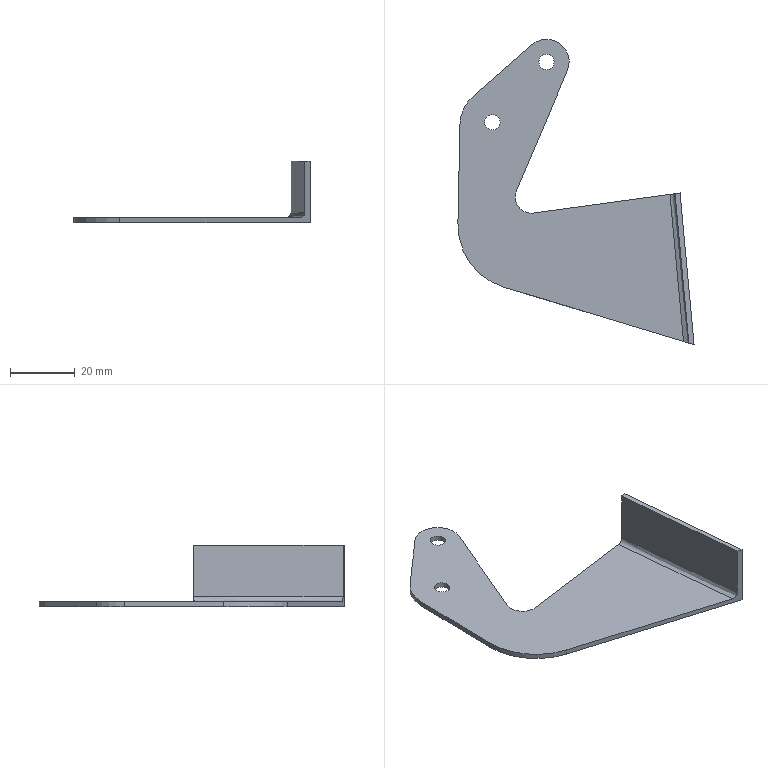Part | NX | features door hinge 2(left) 2 | 1 solid | 17 faces | box 72.898 x 94.256 x 19 mm | volume 6455 mm3 | plane 8 | cylinder 6 | spline 3 | commonest cylinder face diameters 4.762 x1 4.763 x1 10 x1 14 x1 24 x1 40 x1
STEP:
#1=CARTESIAN_POINT('',(6.443,-2.735,1.575));
#2=VERTEX_POINT('',#1);
#3=CARTESIAN_POINT('',(6.443,-2.735,0.));
#4=VERTEX_POINT('',#3);
#5=CARTESIAN_POINT('',(6.443,-2.735,19.));
#6=DIRECTION('',(0.,0.,-1.));
#7=VECTOR('',#6,1000.);
#8=LINE('',#5,#7);
#9=EDGE_CURVE('',#2,#4,#8,.T.);
#10=ORIENTED_EDGE('',*,*,#9,.T.);
#11=CARTESIAN_POINT('',(-4.613,5.265,0.));
#12=VERTEX_POINT('',#11);
#13=CARTESIAN_POINT('',(0.,0.,0.));
#14=DIRECTION('',(0.,0.,1.));
#15=DIRECTION('',(1.,0.,0.));
#16=AXIS2_PLACEMENT_3D('',#13,#14,#15);
#17=CIRCLE('',#16,7.);
#18=EDGE_CURVE('',#4,#12,#17,.T.);
#19=ORIENTED_EDGE('',*,*,#18,.T.);
#20=CARTESIAN_POINT('',(-4.613,5.265,1.575));
#21=VERTEX_POINT('',#20);
#22=CARTESIAN_POINT('',(-4.613,5.265,19.));
#23=DIRECTION('',(0.,0.,-1.));
#24=VECTOR('',#23,1000.);
#25=LINE('',#22,#24);
#26=EDGE_CURVE('',#21,#12,#25,.T.);
#27=ORIENTED_EDGE('',*,*,#26,.F.);
#28=CARTESIAN_POINT('',(0.,0.,1.575));
#29=DIRECTION('',(0.,0.,1.));
#30=DIRECTION('',(1.,0.,0.));
#31=AXIS2_PLACEMENT_3D('',#28,#29,#30);
#32=CIRCLE('',#31,7.);
#33=EDGE_CURVE('',#2,#21,#32,.T.);
#34=ORIENTED_EDGE('',*,*,#33,.F.);
#35=EDGE_LOOP('',(#10,#19,#27,#34));
#36=FACE_BOUND('',#35,.T.);
#37=CARTESIAN_POINT('',(0.,0.,19.));
#38=DIRECTION('',(0.,0.,-1.));
#39=DIRECTION('',(1.,0.,0.));
#40=AXIS2_PLACEMENT_3D('',#37,#38,#39);
#41=CYLINDRICAL_SURFACE('',#40,7.);
#42=ADVANCED_FACE('',(#36),#41,.T.);
#43=CARTESIAN_POINT('',(-9.254,-39.713,1.575));
#44=VERTEX_POINT('',#43);
#45=CARTESIAN_POINT('',(-9.254,-39.713,0.));
#46=VERTEX_POINT('',#45);
#47=CARTESIAN_POINT('',(-9.254,-39.713,19.));
#48=DIRECTION('',(0.,0.,-1.));
#49=VECTOR('',#48,1000.);
#50=LINE('',#47,#49);
#51=EDGE_CURVE('',#44,#46,#50,.T.);
#52=ORIENTED_EDGE('',*,*,#51,.T.);
#53=CARTESIAN_POINT('',(6.443,-2.735,0.));
#54=DIRECTION('',(0.3908,0.9205,0.));
#55=VECTOR('',#54,1000.);
#56=LINE('',#53,#55);
#57=EDGE_CURVE('',#46,#4,#56,.T.);
#58=ORIENTED_EDGE('',*,*,#57,.T.);
#59=ORIENTED_EDGE('',*,*,#9,.F.);
#60=CARTESIAN_POINT('',(6.443,-2.735,1.575));
#61=DIRECTION('',(0.3908,0.9205,0.));
#62=VECTOR('',#61,1000.);
#63=LINE('',#60,#62);
#64=EDGE_CURVE('',#44,#2,#63,.T.);
#65=ORIENTED_EDGE('',*,*,#64,.F.);
#66=EDGE_LOOP('',(#52,#58,#59,#65));
#67=FACE_BOUND('',#66,.T.);
#68=CARTESIAN_POINT('',(6.443,-2.735,19.));
#69=DIRECTION('',(0.9205,-0.3908,0.));
#70=DIRECTION('',(0.3908,0.9205,0.));
#71=AXIS2_PLACEMENT_3D('',#68,#69,#70);
#72=PLANE('',#71);
#73=ADVANCED_FACE('',(#67),#72,.T.);
#74=CARTESIAN_POINT('',(-3.976,-46.621,1.575));
#75=VERTEX_POINT('',#74);
#76=CARTESIAN_POINT('',(-3.976,-46.621,0.));
#77=VERTEX_POINT('',#76);
#78=CARTESIAN_POINT('',(-3.976,-46.621,19.));
#79=DIRECTION('',(0.,0.,-1.));
#80=VECTOR('',#79,1000.);
#81=LINE('',#78,#80);
#82=EDGE_CURVE('',#75,#77,#81,.T.);
#83=ORIENTED_EDGE('',*,*,#82,.T.);
#84=CARTESIAN_POINT('',(-4.652,-41.667,0.));
#85=DIRECTION('',(0.,0.,-1.));
#86=DIRECTION('',(1.,0.,0.));
#87=AXIS2_PLACEMENT_3D('',#84,#85,#86);
#88=CIRCLE('',#87,5.);
#89=EDGE_CURVE('',#77,#46,#88,.T.);
#90=ORIENTED_EDGE('',*,*,#89,.T.);
#91=ORIENTED_EDGE('',*,*,#51,.F.);
#92=CARTESIAN_POINT('',(-4.652,-41.667,1.575));
#93=DIRECTION('',(0.,0.,1.));
#94=DIRECTION('',(1.,0.,0.));
#95=AXIS2_PLACEMENT_3D('',#92,#93,#94);
#96=CIRCLE('',#95,5.);
#97=EDGE_CURVE('',#75,#44,#96,.F.);
#98=ORIENTED_EDGE('',*,*,#97,.F.);
#99=EDGE_LOOP('',(#83,#90,#91,#98));
#100=FACE_BOUND('',#99,.T.);
#101=CARTESIAN_POINT('',(-4.652,-41.667,19.));
#102=DIRECTION('',(0.,0.,-1.));
#103=DIRECTION('',(1.,0.,0.));
#104=AXIS2_PLACEMENT_3D('',#101,#102,#103);
#105=CYLINDRICAL_SURFACE('',#104,5.);
#106=ADVANCED_FACE('',(#100),#105,.F.);
#107=CARTESIAN_POINT('',(39.663,-40.665,19.));
#108=VERTEX_POINT('',#107);
#109=CARTESIAN_POINT('',(39.663,-40.665,3.15));
#110=VERTEX_POINT('',#109);
#111=CARTESIAN_POINT('',(39.663,-40.665,9.5));
#112=DIRECTION('',(0.,0.,-1.));
#113=VECTOR('',#112,1000.);
#114=LINE('',#111,#113);
#115=EDGE_CURVE('',#108,#110,#114,.T.);
#116=ORIENTED_EDGE('',*,*,#115,.F.);
#117=CARTESIAN_POINT('',(41.225,-40.452,19.));
#118=VERTEX_POINT('',#117);
#119=CARTESIAN_POINT('',(-3.976,-46.621,19.));
#120=DIRECTION('',(-0.9908,-0.1352,0.));
#121=VECTOR('',#120,1000.);
#122=LINE('',#119,#121);
#123=EDGE_CURVE('',#118,#108,#122,.T.);
#124=ORIENTED_EDGE('',*,*,#123,.F.);
#125=CARTESIAN_POINT('',(41.225,-40.452,0.));
#126=VERTEX_POINT('',#125);
#127=CARTESIAN_POINT('',(41.225,-40.452,19.));
#128=DIRECTION('',(0.,0.,-1.));
#129=VECTOR('',#128,1000.);
#130=LINE('',#127,#129);
#131=EDGE_CURVE('',#118,#126,#130,.T.);
#132=ORIENTED_EDGE('',*,*,#131,.T.);
#133=CARTESIAN_POINT('',(-3.976,-46.621,0.));
#134=DIRECTION('',(-0.9908,-0.1352,0.));
#135=VECTOR('',#134,1000.);
#136=LINE('',#133,#135);
#137=EDGE_CURVE('',#126,#77,#136,.T.);
#138=ORIENTED_EDGE('',*,*,#137,.T.);
#139=ORIENTED_EDGE('',*,*,#82,.F.);
#140=CARTESIAN_POINT('',(38.101,-40.878,1.575));
#141=VERTEX_POINT('',#140);
#142=CARTESIAN_POINT('',(6.175,-45.236,1.575));
#143=DIRECTION('',(-0.9908,-0.1352,0.));
#144=VECTOR('',#143,1000.);
#145=LINE('',#142,#144);
#146=EDGE_CURVE('',#141,#75,#145,.T.);
#147=ORIENTED_EDGE('',*,*,#146,.F.);
#148=CARTESIAN_POINT('',(39.663,-40.665,3.15));
#149=CARTESIAN_POINT('',(39.663,-40.665,2.317));
#150=CARTESIAN_POINT('',(38.926,-40.765,1.575));
#151=CARTESIAN_POINT('',(38.101,-40.878,1.575));
#152=B_SPLINE_CURVE_WITH_KNOTS('',3,(#148,#149,#150,#151),.UNSPECIFIED.,.F.,.F.,(4,4),(0.,0.002461),.UNSPECIFIED.);
#153=EDGE_CURVE('',#110,#141,#152,.T.);
#154=ORIENTED_EDGE('',*,*,#153,.F.);
#155=EDGE_LOOP('',(#116,#124,#132,#138,#139,#147,#154));
#156=FACE_BOUND('',#155,.T.);
#157=CARTESIAN_POINT('',(-3.976,-46.621,19.));
#158=DIRECTION('',(-0.1352,0.9908,0.));
#159=DIRECTION('',(-0.9908,-0.1352,0.));
#160=AXIS2_PLACEMENT_3D('',#157,#158,#159);
#161=PLANE('',#160);
#162=ADVANCED_FACE('',(#156),#161,.T.);
#163=CARTESIAN_POINT('',(-13.139,-69.495,1.575));
#164=VERTEX_POINT('',#163);
#165=CARTESIAN_POINT('',(-13.139,-69.495,0.));
#166=VERTEX_POINT('',#165);
#167=CARTESIAN_POINT('',(-13.139,-69.495,19.));
#168=DIRECTION('',(0.,0.,-1.));
#169=VECTOR('',#168,1000.);
#170=LINE('',#167,#169);
#171=EDGE_CURVE('',#164,#166,#170,.T.);
#172=ORIENTED_EDGE('',*,*,#171,.T.);
#173=CARTESIAN_POINT('',(45.551,-87.256,0.));
#174=VERTEX_POINT('',#173);
#175=CARTESIAN_POINT('',(45.551,-87.256,0.));
#176=DIRECTION('',(0.9571,-0.2897,0.));
#177=VECTOR('',#176,1000.);
#178=LINE('',#175,#177);
#179=EDGE_CURVE('',#166,#174,#178,.T.);
#180=ORIENTED_EDGE('',*,*,#179,.T.);
#181=CARTESIAN_POINT('',(45.551,-87.256,19.));
#182=VERTEX_POINT('',#181);
#183=CARTESIAN_POINT('',(45.551,-87.256,19.));
#184=DIRECTION('',(0.,0.,-1.));
#185=VECTOR('',#184,1000.);
#186=LINE('',#183,#185);
#187=EDGE_CURVE('',#182,#174,#186,.T.);
#188=ORIENTED_EDGE('',*,*,#187,.F.);
#189=CARTESIAN_POINT('',(43.923,-86.763,19.));
#190=VERTEX_POINT('',#189);
#191=CARTESIAN_POINT('',(45.551,-87.256,19.));
#192=DIRECTION('',(0.9571,-0.2897,0.));
#193=VECTOR('',#192,1000.);
#194=LINE('',#191,#193);
#195=EDGE_CURVE('',#190,#182,#194,.T.);
#196=ORIENTED_EDGE('',*,*,#195,.F.);
#197=CARTESIAN_POINT('',(43.923,-86.763,3.15));
#198=VERTEX_POINT('',#197);
#199=CARTESIAN_POINT('',(43.923,-86.763,9.5));
#200=DIRECTION('',(0.,0.,-1.));
#201=VECTOR('',#200,1000.);
#202=LINE('',#199,#201);
#203=EDGE_CURVE('',#190,#198,#202,.T.);
#204=ORIENTED_EDGE('',*,*,#203,.T.);
#205=CARTESIAN_POINT('',(42.294,-86.27,1.575));
#206=VERTEX_POINT('',#205);
#207=CARTESIAN_POINT('',(42.294,-86.27,1.575));
#208=CARTESIAN_POINT('',(43.123,-86.521,1.575));
#209=CARTESIAN_POINT('',(43.923,-86.763,2.282));
#210=CARTESIAN_POINT('',(43.923,-86.763,3.15));
#211=B_SPLINE_CURVE_WITH_KNOTS('',3,(#207,#208,#209,#210),.UNSPECIFIED.,.F.,.F.,(4,4),(0.,0.00256),.UNSPECIFIED.);
#212=EDGE_CURVE('',#206,#198,#211,.T.);
#213=ORIENTED_EDGE('',*,*,#212,.F.);
#214=CARTESIAN_POINT('',(-20.369,-67.307,1.575));
#215=DIRECTION('',(0.9571,-0.2897,0.));
#216=VECTOR('',#215,1000.);
#217=LINE('',#214,#216);
#218=EDGE_CURVE('',#164,#206,#217,.T.);
#219=ORIENTED_EDGE('',*,*,#218,.F.);
#220=EDGE_LOOP('',(#172,#180,#188,#196,#204,#213,#219));
#221=FACE_BOUND('',#220,.T.);
#222=CARTESIAN_POINT('',(45.551,-87.256,19.));
#223=DIRECTION('',(-0.2897,-0.9571,0.));
#224=DIRECTION('',(0.9571,-0.2897,0.));
#225=AXIS2_PLACEMENT_3D('',#222,#223,#224);
#226=PLANE('',#225);
#227=ADVANCED_FACE('',(#221),#226,.T.);
#228=CARTESIAN_POINT('',(-27.342,-49.937,1.575));
#229=VERTEX_POINT('',#228);
#230=CARTESIAN_POINT('',(-27.342,-49.937,0.));
#231=VERTEX_POINT('',#230);
#232=CARTESIAN_POINT('',(-27.342,-49.937,19.));
#233=DIRECTION('',(0.,0.,-1.));
#234=VECTOR('',#233,1000.);
#235=LINE('',#232,#234);
#236=EDGE_CURVE('',#229,#231,#235,.T.);
#237=ORIENTED_EDGE('',*,*,#236,.T.);
#238=CARTESIAN_POINT('',(-7.346,-50.352,0.));
#239=DIRECTION('',(0.,0.,1.));
#240=DIRECTION('',(1.,0.,0.));
#241=AXIS2_PLACEMENT_3D('',#238,#239,#240);
#242=CIRCLE('',#241,20.);
#243=EDGE_CURVE('',#231,#166,#242,.T.);
#244=ORIENTED_EDGE('',*,*,#243,.T.);
#245=ORIENTED_EDGE('',*,*,#171,.F.);
#246=CARTESIAN_POINT('',(-7.346,-50.352,1.575));
#247=DIRECTION('',(0.,0.,1.));
#248=DIRECTION('',(1.,0.,0.));
#249=AXIS2_PLACEMENT_3D('',#246,#247,#248);
#250=CIRCLE('',#249,20.);
#251=EDGE_CURVE('',#229,#164,#250,.T.);
#252=ORIENTED_EDGE('',*,*,#251,.F.);
#253=EDGE_LOOP('',(#237,#244,#245,#252));
#254=FACE_BOUND('',#253,.T.);
#255=CARTESIAN_POINT('',(-7.346,-50.352,19.));
#256=DIRECTION('',(0.,0.,-1.));
#257=DIRECTION('',(1.,0.,0.));
#258=AXIS2_PLACEMENT_3D('',#255,#256,#257);
#259=CYLINDRICAL_SURFACE('',#258,20.);
#260=ADVANCED_FACE('',(#254),#259,.T.);
#261=CARTESIAN_POINT('',(-26.706,-19.286,0.));
#262=VERTEX_POINT('',#261);
#263=CARTESIAN_POINT('',(-27.342,-49.937,0.));
#264=DIRECTION('',(-0.02074,-0.9998,0.));
#265=VECTOR('',#264,1000.);
#266=LINE('',#263,#265);
#267=EDGE_CURVE('',#262,#231,#266,.T.);
#268=ORIENTED_EDGE('',*,*,#267,.T.);
#269=ORIENTED_EDGE('',*,*,#236,.F.);
#270=CARTESIAN_POINT('',(-26.706,-19.286,1.575));
#271=VERTEX_POINT('',#270);
#272=CARTESIAN_POINT('',(-26.295,0.5454,1.575));
#273=DIRECTION('',(-0.02074,-0.9998,0.));
#274=VECTOR('',#273,1000.);
#275=LINE('',#272,#274);
#276=EDGE_CURVE('',#271,#229,#275,.T.);
#277=ORIENTED_EDGE('',*,*,#276,.F.);
#278=CARTESIAN_POINT('',(-26.706,-19.286,19.));
#279=DIRECTION('',(0.,0.,-1.));
#280=VECTOR('',#279,1000.);
#281=LINE('',#278,#280);
#282=EDGE_CURVE('',#262,#271,#281,.F.);
#283=ORIENTED_EDGE('',*,*,#282,.F.);
#284=EDGE_LOOP('',(#268,#269,#277,#283));
#285=FACE_BOUND('',#284,.T.);
#286=CARTESIAN_POINT('',(-27.342,-49.937,19.));
#287=DIRECTION('',(-0.9998,0.02074,0.));
#288=DIRECTION('',(-0.02074,-0.9998,0.));
#289=AXIS2_PLACEMENT_3D('',#286,#287,#288);
#290=PLANE('',#289);
#291=ADVANCED_FACE('',(#285),#290,.T.);
#292=CARTESIAN_POINT('',(-22.617,-10.509,1.575));
#293=VERTEX_POINT('',#292);
#294=CARTESIAN_POINT('',(-4.613,5.265,1.575));
#295=DIRECTION('',(-0.7521,-0.659,0.));
#296=VECTOR('',#295,1000.);
#297=LINE('',#294,#296);
#298=EDGE_CURVE('',#21,#293,#297,.T.);
#299=ORIENTED_EDGE('',*,*,#298,.F.);
#300=ORIENTED_EDGE('',*,*,#26,.T.);
#301=CARTESIAN_POINT('',(-22.617,-10.509,0.));
#302=VERTEX_POINT('',#301);
#303=CARTESIAN_POINT('',(-26.597,-13.996,0.));
#304=DIRECTION('',(-0.7521,-0.659,0.));
#305=VECTOR('',#304,1000.);
#306=LINE('',#303,#305);
#307=EDGE_CURVE('',#12,#302,#306,.T.);
#308=ORIENTED_EDGE('',*,*,#307,.T.);
#309=CARTESIAN_POINT('',(-22.617,-10.509,19.));
#310=DIRECTION('',(0.,0.,-1.));
#311=VECTOR('',#310,1000.);
#312=LINE('',#309,#311);
#313=EDGE_CURVE('',#293,#302,#312,.T.);
#314=ORIENTED_EDGE('',*,*,#313,.F.);
#315=EDGE_LOOP('',(#299,#300,#308,#314));
#316=FACE_BOUND('',#315,.T.);
#317=CARTESIAN_POINT('',(-26.597,-13.996,19.));
#318=DIRECTION('',(-0.659,0.7521,0.));
#319=DIRECTION('',(-0.7521,-0.659,0.));
#320=AXIS2_PLACEMENT_3D('',#317,#318,#319);
#321=PLANE('',#320);
#322=ADVANCED_FACE('',(#316),#321,.T.);
#323=CARTESIAN_POINT('',(2.381,0.,0.));
#324=VERTEX_POINT('',#323);
#325=CARTESIAN_POINT('',(0.,0.,0.));
#326=DIRECTION('',(0.,0.,1.));
#327=DIRECTION('',(1.,0.,0.));
#328=AXIS2_PLACEMENT_3D('',#325,#326,#327);
#329=CIRCLE('',#328,2.381);
#330=EDGE_CURVE('',#324,#324,#329,.T.);
#331=ORIENTED_EDGE('',*,*,#330,.F.);
#332=EDGE_LOOP('',(#331));
#333=FACE_BOUND('',#332,.T.);
#334=CARTESIAN_POINT('',(2.381,0.,1.575));
#335=VERTEX_POINT('',#334);
#336=CARTESIAN_POINT('',(0.,0.,1.575));
#337=DIRECTION('',(0.,0.,1.));
#338=DIRECTION('',(1.,0.,0.));
#339=AXIS2_PLACEMENT_3D('',#336,#337,#338);
#340=CIRCLE('',#339,2.381);
#341=EDGE_CURVE('',#335,#335,#340,.T.);
#342=ORIENTED_EDGE('',*,*,#341,.T.);
#343=EDGE_LOOP('',(#342));
#344=FACE_BOUND('',#343,.T.);
#345=CARTESIAN_POINT('',(0.,0.,19.));
#346=DIRECTION('',(0.,0.,-1.));
#347=DIRECTION('',(1.,0.,0.));
#348=AXIS2_PLACEMENT_3D('',#345,#346,#347);
#349=CYLINDRICAL_SURFACE('',#348,2.381);
#350=ADVANCED_FACE('',(#333,#344),#349,.F.);
#351=CARTESIAN_POINT('',(-14.309,-18.613,0.));
#352=VERTEX_POINT('',#351);
#353=CARTESIAN_POINT('',(-16.69,-18.613,0.));
#354=DIRECTION('',(0.,0.,1.));
#355=DIRECTION('',(1.,0.,0.));
#356=AXIS2_PLACEMENT_3D('',#353,#354,#355);
#357=CIRCLE('',#356,2.381);
#358=EDGE_CURVE('',#352,#352,#357,.T.);
#359=ORIENTED_EDGE('',*,*,#358,.F.);
#360=EDGE_LOOP('',(#359));
#361=FACE_BOUND('',#360,.T.);
#362=CARTESIAN_POINT('',(-14.309,-18.613,1.575));
#363=VERTEX_POINT('',#362);
#364=CARTESIAN_POINT('',(-16.69,-18.613,1.575));
#365=DIRECTION('',(0.,0.,1.));
#366=DIRECTION('',(1.,0.,0.));
#367=AXIS2_PLACEMENT_3D('',#364,#365,#366);
#368=CIRCLE('',#367,2.381);
#369=EDGE_CURVE('',#363,#363,#368,.T.);
#370=ORIENTED_EDGE('',*,*,#369,.T.);
#371=EDGE_LOOP('',(#370));
#372=FACE_BOUND('',#371,.T.);
#373=CARTESIAN_POINT('',(-16.69,-18.613,19.));
#374=DIRECTION('',(0.,0.,-1.));
#375=DIRECTION('',(1.,0.,0.));
#376=AXIS2_PLACEMENT_3D('',#373,#374,#375);
#377=CYLINDRICAL_SURFACE('',#376,2.381);
#378=ADVANCED_FACE('',(#361,#372),#377,.F.);
#379=CARTESIAN_POINT('',(45.551,-87.256,0.));
#380=CARTESIAN_POINT('',(44.075,-71.658,0.));
#381=CARTESIAN_POINT('',(42.633,-56.056,0.));
#382=CARTESIAN_POINT('',(41.225,-40.452,0.));
#383=B_SPLINE_CURVE_WITH_KNOTS('',3,(#379,#380,#381,#382),.UNSPECIFIED.,.F.,.F.,(4,4),(2.331,49.335),.PIECEWISE_BEZIER_KNOTS.);
#384=EDGE_CURVE('',#174,#126,#383,.T.);
#385=ORIENTED_EDGE('',*,*,#384,.T.);
#386=ORIENTED_EDGE('',*,*,#131,.F.);
#387=CARTESIAN_POINT('',(45.551,-87.256,19.));
#388=CARTESIAN_POINT('',(44.075,-71.658,19.));
#389=CARTESIAN_POINT('',(42.633,-56.056,19.));
#390=CARTESIAN_POINT('',(41.225,-40.452,19.));
#391=B_SPLINE_CURVE_WITH_KNOTS('',3,(#387,#388,#389,#390),.UNSPECIFIED.,.F.,.F.,(4,4),(2.331,49.335),.PIECEWISE_BEZIER_KNOTS.);
#392=EDGE_CURVE('',#182,#118,#391,.T.);
#393=ORIENTED_EDGE('',*,*,#392,.F.);
#394=ORIENTED_EDGE('',*,*,#187,.T.);
#395=EDGE_LOOP('',(#385,#386,#393,#394));
#396=FACE_BOUND('',#395,.T.);
#397=CARTESIAN_POINT('',(45.551,-87.256,19.));
#398=CARTESIAN_POINT('',(45.551,-87.256,0.));
#399=CARTESIAN_POINT('',(44.075,-71.658,19.));
#400=CARTESIAN_POINT('',(44.075,-71.658,0.));
#401=CARTESIAN_POINT('',(42.633,-56.056,19.));
#402=CARTESIAN_POINT('',(42.633,-56.056,0.));
#403=CARTESIAN_POINT('',(41.225,-40.452,19.));
#404=CARTESIAN_POINT('',(41.225,-40.452,0.));
#405=B_SPLINE_SURFACE_WITH_KNOTS('',3,1,((#397,#398),(#399,#400),(#401,#402),(#403,#404)),.SURF_OF_LINEAR_EXTRUSION.,.F.,.F.,.F.,(4,4),(2,2),(2.331,49.335),(0.,1.),.PIECEWISE_BEZIER_KNOTS.);
#406=ADVANCED_FACE('',(#396),#405,.F.);
#407=ORIENTED_EDGE('',*,*,#195,.T.);
#408=ORIENTED_EDGE('',*,*,#392,.T.);
#409=ORIENTED_EDGE('',*,*,#123,.T.);
#410=CARTESIAN_POINT('',(43.923,-86.763,19.));
#411=CARTESIAN_POINT('',(42.469,-71.4,19.));
#412=CARTESIAN_POINT('',(41.05,-56.034,19.));
#413=CARTESIAN_POINT('',(39.663,-40.665,19.));
#414=B_SPLINE_CURVE_WITH_KNOTS('',3,(#410,#411,#412,#413),.UNSPECIFIED.,.F.,.F.,(4,4),(0.,0.04629),.UNSPECIFIED.);
#415=EDGE_CURVE('',#190,#108,#414,.T.);
#416=ORIENTED_EDGE('',*,*,#415,.F.);
#417=EDGE_LOOP('',(#407,#408,#409,#416));
#418=FACE_BOUND('',#417,.T.);
#419=CARTESIAN_POINT('',(0.,0.,19.));
#420=DIRECTION('',(0.,0.,-1.));
#421=DIRECTION('',(1.,0.,0.));
#422=AXIS2_PLACEMENT_3D('',#419,#420,#421);
#423=PLANE('',#422);
#424=ADVANCED_FACE('',(#418),#423,.F.);
#425=ORIENTED_EDGE('',*,*,#358,.T.);
#426=EDGE_LOOP('',(#425));
#427=FACE_BOUND('',#426,.T.);
#428=ORIENTED_EDGE('',*,*,#330,.T.);
#429=EDGE_LOOP('',(#428));
#430=FACE_BOUND('',#429,.T.);
#431=ORIENTED_EDGE('',*,*,#307,.F.);
#432=ORIENTED_EDGE('',*,*,#18,.F.);
#433=ORIENTED_EDGE('',*,*,#57,.F.);
#434=ORIENTED_EDGE('',*,*,#89,.F.);
#435=ORIENTED_EDGE('',*,*,#137,.F.);
#436=ORIENTED_EDGE('',*,*,#384,.F.);
#437=ORIENTED_EDGE('',*,*,#179,.F.);
#438=ORIENTED_EDGE('',*,*,#243,.F.);
#439=ORIENTED_EDGE('',*,*,#267,.F.);
#440=CARTESIAN_POINT('',(-14.709,-19.535,0.));
#441=DIRECTION('',(0.,0.,1.));
#442=DIRECTION('',(1.,0.,0.));
#443=AXIS2_PLACEMENT_3D('',#440,#441,#442);
#444=CIRCLE('',#443,12.);
#445=EDGE_CURVE('',#302,#262,#444,.T.);
#446=ORIENTED_EDGE('',*,*,#445,.F.);
#447=EDGE_LOOP('',(#431,#432,#433,#434,#435,#436,#437,#438,#439,#446));
#448=FACE_BOUND('',#447,.T.);
#449=CARTESIAN_POINT('',(0.,0.,0.));
#450=DIRECTION('',(0.,0.,-1.));
#451=DIRECTION('',(1.,0.,0.));
#452=AXIS2_PLACEMENT_3D('',#449,#450,#451);
#453=PLANE('',#452);
#454=ADVANCED_FACE('',(#427,#430,#448),#453,.T.);
#455=ORIENTED_EDGE('',*,*,#203,.F.);
#456=ORIENTED_EDGE('',*,*,#415,.T.);
#457=ORIENTED_EDGE('',*,*,#115,.T.);
#458=CARTESIAN_POINT('',(43.923,-86.763,3.15));
#459=CARTESIAN_POINT('',(42.469,-71.4,3.15));
#460=CARTESIAN_POINT('',(41.05,-56.034,3.15));
#461=CARTESIAN_POINT('',(39.663,-40.665,3.15));
#462=B_SPLINE_CURVE_WITH_KNOTS('',3,(#458,#459,#460,#461),.UNSPECIFIED.,.F.,.F.,(4,4),(0.,0.04629),.UNSPECIFIED.);
#463=EDGE_CURVE('',#198,#110,#462,.T.);
#464=ORIENTED_EDGE('',*,*,#463,.F.);
#465=EDGE_LOOP('',(#455,#456,#457,#464));
#466=FACE_BOUND('',#465,.T.);
#467=CARTESIAN_POINT('',(43.923,-86.763,19.));
#468=CARTESIAN_POINT('',(43.923,-86.763,3.15));
#469=CARTESIAN_POINT('',(42.469,-71.4,19.));
#470=CARTESIAN_POINT('',(42.469,-71.4,3.15));
#471=CARTESIAN_POINT('',(41.05,-56.034,19.));
#472=CARTESIAN_POINT('',(41.05,-56.034,3.15));
#473=CARTESIAN_POINT('',(39.663,-40.665,19.));
#474=CARTESIAN_POINT('',(39.663,-40.665,3.15));
#475=B_SPLINE_SURFACE_WITH_KNOTS('',3,1,((#467,#468),(#469,#470),(#471,#472),(#473,#474)),.SURF_OF_LINEAR_EXTRUSION.,.F.,.F.,.F.,(4,4),(2,2),(2.975,49.263),(0.,1.),.PIECEWISE_BEZIER_KNOTS.);
#476=ADVANCED_FACE('',(#466),#475,.T.);
#477=ORIENTED_EDGE('',*,*,#369,.F.);
#478=EDGE_LOOP('',(#477));
#479=FACE_BOUND('',#478,.T.);
#480=ORIENTED_EDGE('',*,*,#341,.F.);
#481=EDGE_LOOP('',(#480));
#482=FACE_BOUND('',#481,.T.);
#483=ORIENTED_EDGE('',*,*,#146,.T.);
#484=ORIENTED_EDGE('',*,*,#97,.T.);
#485=ORIENTED_EDGE('',*,*,#64,.T.);
#486=ORIENTED_EDGE('',*,*,#33,.T.);
#487=ORIENTED_EDGE('',*,*,#298,.T.);
#488=CARTESIAN_POINT('',(-14.709,-19.535,1.575));
#489=DIRECTION('',(0.,0.,1.));
#490=DIRECTION('',(1.,0.,0.));
#491=AXIS2_PLACEMENT_3D('',#488,#489,#490);
#492=CIRCLE('',#491,12.);
#493=EDGE_CURVE('',#271,#293,#492,.F.);
#494=ORIENTED_EDGE('',*,*,#493,.F.);
#495=ORIENTED_EDGE('',*,*,#276,.T.);
#496=ORIENTED_EDGE('',*,*,#251,.T.);
#497=ORIENTED_EDGE('',*,*,#218,.T.);
#498=CARTESIAN_POINT('',(38.101,-40.878,1.575));
#499=CARTESIAN_POINT('',(39.467,-56.012,1.575));
#500=CARTESIAN_POINT('',(40.864,-71.142,1.575));
#501=CARTESIAN_POINT('',(42.294,-86.27,1.575));
#502=B_SPLINE_CURVE_WITH_KNOTS('',3,(#498,#499,#500,#501),.UNSPECIFIED.,.F.,.F.,(4,4),(0.,0.04559),.UNSPECIFIED.);
#503=EDGE_CURVE('',#141,#206,#502,.T.);
#504=ORIENTED_EDGE('',*,*,#503,.F.);
#505=EDGE_LOOP('',(#483,#484,#485,#486,#487,#494,#495,#496,#497,#504));
#506=FACE_BOUND('',#505,.T.);
#507=CARTESIAN_POINT('',(0.,0.,1.575));
#508=DIRECTION('',(0.,0.,-1.));
#509=DIRECTION('',(1.,0.,0.));
#510=AXIS2_PLACEMENT_3D('',#507,#508,#509);
#511=PLANE('',#510);
#512=ADVANCED_FACE('',(#479,#482,#506),#511,.F.);
#513=ORIENTED_EDGE('',*,*,#493,.T.);
#514=ORIENTED_EDGE('',*,*,#313,.T.);
#515=ORIENTED_EDGE('',*,*,#445,.T.);
#516=ORIENTED_EDGE('',*,*,#282,.T.);
#517=EDGE_LOOP('',(#513,#514,#515,#516));
#518=FACE_BOUND('',#517,.T.);
#519=CARTESIAN_POINT('',(-14.709,-19.535,19.));
#520=DIRECTION('',(0.,0.,-1.));
#521=DIRECTION('',(1.,0.,0.));
#522=AXIS2_PLACEMENT_3D('',#519,#520,#521);
#523=CYLINDRICAL_SURFACE('',#522,12.);
#524=ADVANCED_FACE('',(#518),#523,.T.);
#525=ORIENTED_EDGE('',*,*,#212,.T.);
#526=ORIENTED_EDGE('',*,*,#463,.T.);
#527=ORIENTED_EDGE('',*,*,#153,.T.);
#528=ORIENTED_EDGE('',*,*,#503,.T.);
#529=EDGE_LOOP('',(#525,#526,#527,#528));
#530=FACE_BOUND('',#529,.T.);
#531=CARTESIAN_POINT('',(42.381,-87.188,1.575));
#532=CARTESIAN_POINT('',(43.949,-87.04,1.575));
#533=CARTESIAN_POINT('',(43.949,-87.04,3.15));
#534=CARTESIAN_POINT('',(40.91,-71.638,1.575));
#535=CARTESIAN_POINT('',(42.478,-71.492,1.575));
#536=CARTESIAN_POINT('',(42.478,-71.492,3.15));
#537=CARTESIAN_POINT('',(39.473,-56.085,1.575));
#538=CARTESIAN_POINT('',(41.041,-55.944,1.575));
#539=CARTESIAN_POINT('',(41.041,-55.944,3.15));
#540=CARTESIAN_POINT('',(38.07,-40.53,1.575));
#541=CARTESIAN_POINT('',(39.638,-40.388,1.575));
#542=CARTESIAN_POINT('',(39.638,-40.388,3.15));
#543=(BOUNDED_SURFACE()B_SPLINE_SURFACE(3,2,((#531,#532,#533),(#534,#535,#536),(#537,#538,#539),(#540,#541,#542)),.UNSPECIFIED.,.F.,.F.,.F.)B_SPLINE_SURFACE_WITH_KNOTS((4,4),(3,3),(0.01148,0.05833),(0.,1.),.PIECEWISE_BEZIER_KNOTS.)GEOMETRIC_REPRESENTATION_ITEM()RATIONAL_B_SPLINE_SURFACE(((1.,0.7071,1.),(1.,0.7071,1.),(1.,0.7071,1.),(1.,0.7071,1.)))REPRESENTATION_ITEM('')SURFACE());
#544=ADVANCED_FACE('',(#530),#543,.F.);
#545=CLOSED_SHELL('',(#42,#73,#106,#162,#227,#260,#291,#322,#350,#378,#406,#424,#454,#476,#512,#524,#544));
#546=MANIFOLD_SOLID_BREP('',#545);
#547=(LENGTH_UNIT()NAMED_UNIT(*)SI_UNIT(.MILLI.,.METRE.));
#548=UNCERTAINTY_MEASURE_WITH_UNIT(LENGTH_MEASURE(0.0508),#547,'','');
#549=(NAMED_UNIT(*)PLANE_ANGLE_UNIT()SI_UNIT($,.RADIAN.));
#550=(NAMED_UNIT(*)SI_UNIT($,.STERADIAN.)SOLID_ANGLE_UNIT());
#551=(GEOMETRIC_REPRESENTATION_CONTEXT(3)GLOBAL_UNCERTAINTY_ASSIGNED_CONTEXT((#548))GLOBAL_UNIT_ASSIGNED_CONTEXT((#547,#549,#550))REPRESENTATION_CONTEXT('',''));
#552=ADVANCED_BREP_SHAPE_REPRESENTATION('',(#546),#551);